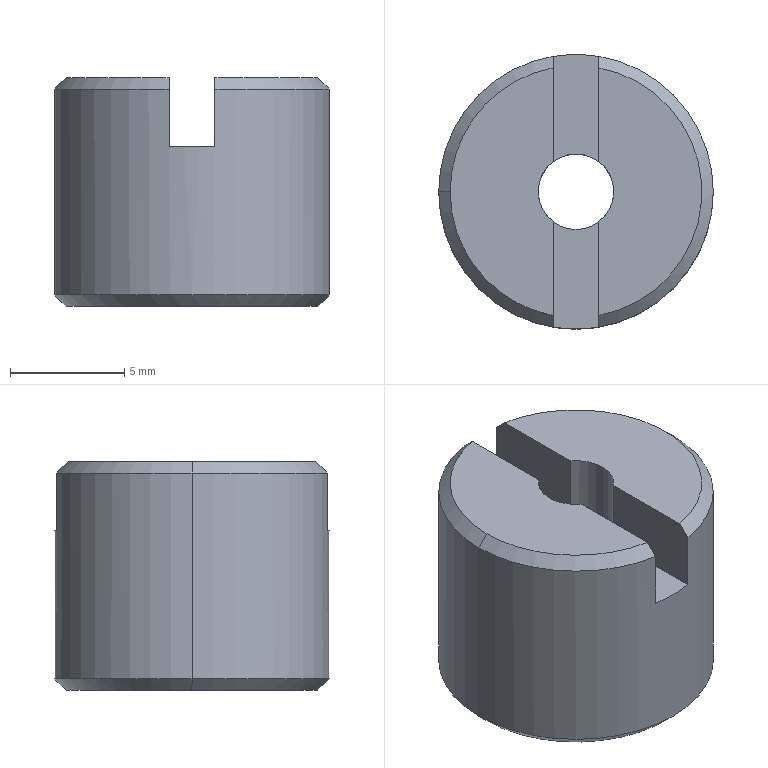Part | STEP file | PN_0004 | 1 solid | 23 faces | box 12 x 12 x 10 mm | volume 792.649 mm3 | plane 10 | cone 7 | cylinder 6 | commonest cylinder face diameters 3.3 x2 8 x2 12 x2